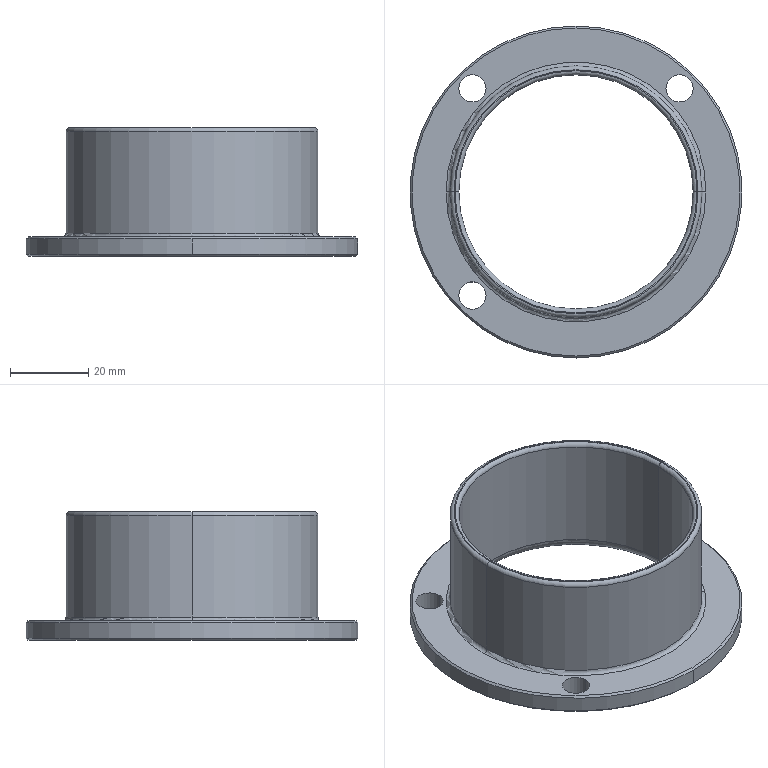Part | NX | features solid 2 | 1 solid | 27 faces | box 85 x 85 x 33 mm | volume 25500 mm3 | cylinder 12 | torus 8 | cone 4 | plane 3 | commonest cylinder face diameters 7 x6 60 x2 64.5 x2 85 x2
STEP:
#1=CARTESIAN_POINT('',(-450.,-1677.,947.));
#2=VERTEX_POINT('',#1);
#3=CARTESIAN_POINT('',(-450.,-1677.5,947.5));
#4=VERTEX_POINT('',#3);
#5=CARTESIAN_POINT('',(-450.,-1677.,947.));
#6=DIRECTION('',(0.,-0.7071,0.7071));
#7=VECTOR('',#6,1000.);
#8=LINE('',#5,#7);
#9=EDGE_CURVE('',#2,#4,#8,.T.);
#10=ORIENTED_EDGE('',*,*,#9,.F.);
#11=CARTESIAN_POINT('',(-450.,-1593.,947.));
#12=VERTEX_POINT('',#11);
#13=CARTESIAN_POINT('',(-450.,-1635.,947.));
#14=DIRECTION('',(0.,0.,-1.));
#15=DIRECTION('',(-1.,0.,0.));
#16=AXIS2_PLACEMENT_3D('',#13,#14,#15);
#17=CIRCLE('',#16,42.);
#18=EDGE_CURVE('',#12,#2,#17,.T.);
#19=ORIENTED_EDGE('',*,*,#18,.F.);
#20=CARTESIAN_POINT('',(-450.,-1592.5,947.5));
#21=VERTEX_POINT('',#20);
#22=CARTESIAN_POINT('',(-450.,-1593.,947.));
#23=DIRECTION('',(0.,0.7071,0.7071));
#24=VECTOR('',#23,1000.);
#25=LINE('',#22,#24);
#26=EDGE_CURVE('',#21,#12,#25,.F.);
#27=ORIENTED_EDGE('',*,*,#26,.F.);
#28=CARTESIAN_POINT('',(-450.,-1635.,947.5));
#29=DIRECTION('',(0.,0.,1.));
#30=DIRECTION('',(0.,-1.,0.));
#31=AXIS2_PLACEMENT_3D('',#28,#29,#30);
#32=CIRCLE('',#31,42.5);
#33=EDGE_CURVE('',#4,#21,#32,.T.);
#34=ORIENTED_EDGE('',*,*,#33,.F.);
#35=EDGE_LOOP('',(#10,#19,#27,#34));
#36=FACE_BOUND('',#35,.T.);
#37=CARTESIAN_POINT('',(-450.,-1635.,947.));
#38=DIRECTION('',(0.,0.,1.));
#39=DIRECTION('',(0.,1.,0.));
#40=AXIS2_PLACEMENT_3D('',#37,#38,#39);
#41=CONICAL_SURFACE('',#40,42.,0.7854);
#42=ADVANCED_FACE('',(#36),#41,.T.);
#43=CARTESIAN_POINT('',(-450.,-1593.,952.));
#44=VERTEX_POINT('',#43);
#45=CARTESIAN_POINT('',(-450.,-1592.5,951.5));
#46=VERTEX_POINT('',#45);
#47=CARTESIAN_POINT('',(-450.,-1592.5,951.5));
#48=DIRECTION('',(0.,0.7071,-0.7071));
#49=VECTOR('',#48,1000.);
#50=LINE('',#47,#49);
#51=EDGE_CURVE('',#44,#46,#50,.T.);
#52=ORIENTED_EDGE('',*,*,#51,.F.);
#53=CARTESIAN_POINT('',(-450.,-1677.,952.));
#54=VERTEX_POINT('',#53);
#55=CARTESIAN_POINT('',(-450.,-1635.,952.));
#56=DIRECTION('',(0.,0.,1.));
#57=DIRECTION('',(-1.,0.,0.));
#58=AXIS2_PLACEMENT_3D('',#55,#56,#57);
#59=CIRCLE('',#58,42.);
#60=EDGE_CURVE('',#54,#44,#59,.T.);
#61=ORIENTED_EDGE('',*,*,#60,.F.);
#62=CARTESIAN_POINT('',(-450.,-1677.5,951.5));
#63=VERTEX_POINT('',#62);
#64=CARTESIAN_POINT('',(-450.,-1677.5,951.5));
#65=DIRECTION('',(0.,-0.7071,-0.7071));
#66=VECTOR('',#65,1000.);
#67=LINE('',#64,#66);
#68=EDGE_CURVE('',#63,#54,#67,.F.);
#69=ORIENTED_EDGE('',*,*,#68,.F.);
#70=CARTESIAN_POINT('',(-450.,-1635.,951.5));
#71=DIRECTION('',(0.,0.,-1.));
#72=DIRECTION('',(0.,-1.,0.));
#73=AXIS2_PLACEMENT_3D('',#70,#71,#72);
#74=CIRCLE('',#73,42.5);
#75=EDGE_CURVE('',#46,#63,#74,.T.);
#76=ORIENTED_EDGE('',*,*,#75,.F.);
#77=EDGE_LOOP('',(#52,#61,#69,#76));
#78=FACE_BOUND('',#77,.T.);
#79=CARTESIAN_POINT('',(-450.,-1635.,951.5));
#80=DIRECTION('',(0.,0.,-1.));
#81=DIRECTION('',(0.,-1.,0.));
#82=AXIS2_PLACEMENT_3D('',#79,#80,#81);
#83=CONICAL_SURFACE('',#82,42.5,0.7854);
#84=ADVANCED_FACE('',(#78),#83,.T.);
#85=CARTESIAN_POINT('',(-417.75,-1635.,979.));
#86=VERTEX_POINT('',#85);
#87=CARTESIAN_POINT('',(-418.75,-1635.,980.));
#88=VERTEX_POINT('',#87);
#89=CARTESIAN_POINT('',(-418.75,-1635.,979.));
#90=DIRECTION('',(0.,1.,0.));
#91=DIRECTION('',(0.,0.,1.));
#92=AXIS2_PLACEMENT_3D('',#89,#90,#91);
#93=CIRCLE('',#92,1.);
#94=EDGE_CURVE('',#86,#88,#93,.F.);
#95=ORIENTED_EDGE('',*,*,#94,.T.);
#96=CARTESIAN_POINT('',(-481.25,-1635.,980.));
#97=VERTEX_POINT('',#96);
#98=CARTESIAN_POINT('',(-450.,-1635.,980.));
#99=DIRECTION('',(0.,0.,1.));
#100=DIRECTION('',(-1.,0.,0.));
#101=AXIS2_PLACEMENT_3D('',#98,#99,#100);
#102=CIRCLE('',#101,31.25);
#103=EDGE_CURVE('',#97,#88,#102,.T.);
#104=ORIENTED_EDGE('',*,*,#103,.F.);
#105=CARTESIAN_POINT('',(-482.25,-1635.,979.));
#106=VERTEX_POINT('',#105);
#107=CARTESIAN_POINT('',(-481.25,-1635.,979.));
#108=DIRECTION('',(0.,-1.,0.));
#109=DIRECTION('',(0.,0.,-1.));
#110=AXIS2_PLACEMENT_3D('',#107,#108,#109);
#111=CIRCLE('',#110,1.);
#112=EDGE_CURVE('',#97,#106,#111,.T.);
#113=ORIENTED_EDGE('',*,*,#112,.T.);
#114=CARTESIAN_POINT('',(-450.,-1635.,979.));
#115=DIRECTION('',(0.,0.,-1.));
#116=DIRECTION('',(-1.,0.,0.));
#117=AXIS2_PLACEMENT_3D('',#114,#115,#116);
#118=CIRCLE('',#117,32.25);
#119=EDGE_CURVE('',#86,#106,#118,.T.);
#120=ORIENTED_EDGE('',*,*,#119,.F.);
#121=EDGE_LOOP('',(#95,#104,#113,#120));
#122=FACE_BOUND('',#121,.T.);
#123=CARTESIAN_POINT('',(-450.,-1635.,979.));
#124=DIRECTION('',(0.,0.,-1.));
#125=DIRECTION('',(-1.,0.,0.));
#126=AXIS2_PLACEMENT_3D('',#123,#124,#125);
#127=TOROIDAL_SURFACE('',#126,31.25,1.);
#128=ADVANCED_FACE('',(#122),#127,.T.);
#129=CARTESIAN_POINT('',(-419.,-1635.,980.));
#130=VERTEX_POINT('',#129);
#131=CARTESIAN_POINT('',(-420.,-1635.,979.));
#132=VERTEX_POINT('',#131);
#133=CARTESIAN_POINT('',(-419.,-1635.,979.));
#134=DIRECTION('',(0.,1.,0.));
#135=DIRECTION('',(0.,0.,1.));
#136=AXIS2_PLACEMENT_3D('',#133,#134,#135);
#137=CIRCLE('',#136,1.);
#138=EDGE_CURVE('',#130,#132,#137,.F.);
#139=ORIENTED_EDGE('',*,*,#138,.T.);
#140=CARTESIAN_POINT('',(-480.,-1635.,979.));
#141=VERTEX_POINT('',#140);
#142=CARTESIAN_POINT('',(-450.,-1635.,979.));
#143=DIRECTION('',(0.,0.,1.));
#144=DIRECTION('',(-1.,0.,0.));
#145=AXIS2_PLACEMENT_3D('',#142,#143,#144);
#146=CIRCLE('',#145,30.);
#147=EDGE_CURVE('',#141,#132,#146,.T.);
#148=ORIENTED_EDGE('',*,*,#147,.F.);
#149=CARTESIAN_POINT('',(-481.,-1635.,980.));
#150=VERTEX_POINT('',#149);
#151=CARTESIAN_POINT('',(-481.,-1635.,979.));
#152=DIRECTION('',(0.,-1.,0.));
#153=DIRECTION('',(0.,0.,-1.));
#154=AXIS2_PLACEMENT_3D('',#151,#152,#153);
#155=CIRCLE('',#154,1.);
#156=EDGE_CURVE('',#141,#150,#155,.T.);
#157=ORIENTED_EDGE('',*,*,#156,.T.);
#158=CARTESIAN_POINT('',(-450.,-1635.,980.));
#159=DIRECTION('',(0.,0.,-1.));
#160=DIRECTION('',(-1.,0.,0.));
#161=AXIS2_PLACEMENT_3D('',#158,#159,#160);
#162=CIRCLE('',#161,31.);
#163=EDGE_CURVE('',#130,#150,#162,.T.);
#164=ORIENTED_EDGE('',*,*,#163,.F.);
#165=EDGE_LOOP('',(#139,#148,#157,#164));
#166=FACE_BOUND('',#165,.T.);
#167=CARTESIAN_POINT('',(-450.,-1635.,979.));
#168=DIRECTION('',(0.,0.,-1.));
#169=DIRECTION('',(-1.,0.,0.));
#170=AXIS2_PLACEMENT_3D('',#167,#168,#169);
#171=TOROIDAL_SURFACE('',#170,31.,1.);
#172=ADVANCED_FACE('',(#166),#171,.T.);
#173=CARTESIAN_POINT('',(-416.75,-1635.,952.));
#174=VERTEX_POINT('',#173);
#175=CARTESIAN_POINT('',(-417.75,-1635.,953.));
#176=VERTEX_POINT('',#175);
#177=CARTESIAN_POINT('',(-416.75,-1635.,953.));
#178=DIRECTION('',(0.,1.,0.));
#179=DIRECTION('',(0.,0.,1.));
#180=AXIS2_PLACEMENT_3D('',#177,#178,#179);
#181=CIRCLE('',#180,1.);
#182=EDGE_CURVE('',#174,#176,#181,.T.);
#183=ORIENTED_EDGE('',*,*,#182,.F.);
#184=CARTESIAN_POINT('',(-483.25,-1635.,952.));
#185=VERTEX_POINT('',#184);
#186=CARTESIAN_POINT('',(-450.,-1635.,952.));
#187=DIRECTION('',(0.,0.,-1.));
#188=DIRECTION('',(-1.,0.,0.));
#189=AXIS2_PLACEMENT_3D('',#186,#187,#188);
#190=CIRCLE('',#189,33.25);
#191=EDGE_CURVE('',#185,#174,#190,.T.);
#192=ORIENTED_EDGE('',*,*,#191,.F.);
#193=CARTESIAN_POINT('',(-482.25,-1635.,953.));
#194=VERTEX_POINT('',#193);
#195=CARTESIAN_POINT('',(-483.25,-1635.,953.));
#196=DIRECTION('',(0.,-1.,0.));
#197=DIRECTION('',(0.,0.,-1.));
#198=AXIS2_PLACEMENT_3D('',#195,#196,#197);
#199=CIRCLE('',#198,1.);
#200=EDGE_CURVE('',#194,#185,#199,.F.);
#201=ORIENTED_EDGE('',*,*,#200,.F.);
#202=CARTESIAN_POINT('',(-450.,-1635.,953.));
#203=DIRECTION('',(0.,0.,1.));
#204=DIRECTION('',(-1.,0.,0.));
#205=AXIS2_PLACEMENT_3D('',#202,#203,#204);
#206=CIRCLE('',#205,32.25);
#207=EDGE_CURVE('',#176,#194,#206,.T.);
#208=ORIENTED_EDGE('',*,*,#207,.F.);
#209=EDGE_LOOP('',(#183,#192,#201,#208));
#210=FACE_BOUND('',#209,.T.);
#211=CARTESIAN_POINT('',(-450.,-1635.,953.));
#212=DIRECTION('',(0.,0.,-1.));
#213=DIRECTION('',(-1.,0.,0.));
#214=AXIS2_PLACEMENT_3D('',#211,#212,#213);
#215=TOROIDAL_SURFACE('',#214,33.25,1.);
#216=ADVANCED_FACE('',(#210),#215,.F.);
#217=CARTESIAN_POINT('',(-420.,-1635.,950.));
#218=VERTEX_POINT('',#217);
#219=CARTESIAN_POINT('',(-417.,-1635.,947.));
#220=VERTEX_POINT('',#219);
#221=CARTESIAN_POINT('',(-417.,-1635.,950.));
#222=DIRECTION('',(0.,1.,0.));
#223=DIRECTION('',(0.,0.,1.));
#224=AXIS2_PLACEMENT_3D('',#221,#222,#223);
#225=CIRCLE('',#224,3.);
#226=EDGE_CURVE('',#218,#220,#225,.F.);
#227=ORIENTED_EDGE('',*,*,#226,.T.);
#228=CARTESIAN_POINT('',(-483.,-1635.,947.));
#229=VERTEX_POINT('',#228);
#230=CARTESIAN_POINT('',(-450.,-1635.,947.));
#231=DIRECTION('',(0.,0.,1.));
#232=DIRECTION('',(-1.,0.,0.));
#233=AXIS2_PLACEMENT_3D('',#230,#231,#232);
#234=CIRCLE('',#233,33.);
#235=EDGE_CURVE('',#229,#220,#234,.T.);
#236=ORIENTED_EDGE('',*,*,#235,.F.);
#237=CARTESIAN_POINT('',(-480.,-1635.,950.));
#238=VERTEX_POINT('',#237);
#239=CARTESIAN_POINT('',(-483.,-1635.,950.));
#240=DIRECTION('',(0.,-1.,0.));
#241=DIRECTION('',(0.,0.,-1.));
#242=AXIS2_PLACEMENT_3D('',#239,#240,#241);
#243=CIRCLE('',#242,3.);
#244=EDGE_CURVE('',#229,#238,#243,.T.);
#245=ORIENTED_EDGE('',*,*,#244,.T.);
#246=CARTESIAN_POINT('',(-450.,-1635.,950.));
#247=DIRECTION('',(0.,0.,-1.));
#248=DIRECTION('',(-1.,0.,0.));
#249=AXIS2_PLACEMENT_3D('',#246,#247,#248);
#250=CIRCLE('',#249,30.);
#251=EDGE_CURVE('',#218,#238,#250,.T.);
#252=ORIENTED_EDGE('',*,*,#251,.F.);
#253=EDGE_LOOP('',(#227,#236,#245,#252));
#254=FACE_BOUND('',#253,.T.);
#255=CARTESIAN_POINT('',(-450.,-1635.,950.));
#256=DIRECTION('',(0.,0.,-1.));
#257=DIRECTION('',(-1.,0.,0.));
#258=AXIS2_PLACEMENT_3D('',#255,#256,#257);
#259=TOROIDAL_SURFACE('',#258,33.,3.);
#260=ADVANCED_FACE('',(#254),#259,.T.);
#261=CARTESIAN_POINT('',(-426.983,-1608.483,952.));
#262=VERTEX_POINT('',#261);
#263=CARTESIAN_POINT('',(-426.983,-1608.483,947.));
#264=VERTEX_POINT('',#263);
#265=CARTESIAN_POINT('',(-426.983,-1608.483,827.344));
#266=DIRECTION('',(0.,0.,1.));
#267=VECTOR('',#266,1000.);
#268=LINE('',#265,#267);
#269=EDGE_CURVE('',#262,#264,#268,.F.);
#270=ORIENTED_EDGE('',*,*,#269,.T.);
#271=CARTESIAN_POINT('',(-419.983,-1608.483,947.));
#272=VERTEX_POINT('',#271);
#273=CARTESIAN_POINT('',(-423.483,-1608.483,947.));
#274=DIRECTION('',(0.,0.,-1.));
#275=DIRECTION('',(-1.,0.,0.));
#276=AXIS2_PLACEMENT_3D('',#273,#274,#275);
#277=CIRCLE('',#276,3.5);
#278=EDGE_CURVE('',#264,#272,#277,.T.);
#279=ORIENTED_EDGE('',*,*,#278,.T.);
#280=CARTESIAN_POINT('',(-419.983,-1608.483,952.));
#281=VERTEX_POINT('',#280);
#282=CARTESIAN_POINT('',(-419.983,-1608.483,827.344));
#283=DIRECTION('',(0.,0.,1.));
#284=VECTOR('',#283,1000.);
#285=LINE('',#282,#284);
#286=EDGE_CURVE('',#272,#281,#285,.T.);
#287=ORIENTED_EDGE('',*,*,#286,.T.);
#288=CARTESIAN_POINT('',(-423.483,-1608.483,952.));
#289=DIRECTION('',(0.,0.,1.));
#290=DIRECTION('',(0.,1.,0.));
#291=AXIS2_PLACEMENT_3D('',#288,#289,#290);
#292=CIRCLE('',#291,3.5);
#293=EDGE_CURVE('',#281,#262,#292,.T.);
#294=ORIENTED_EDGE('',*,*,#293,.T.);
#295=EDGE_LOOP('',(#270,#279,#287,#294));
#296=FACE_BOUND('',#295,.T.);
#297=CARTESIAN_POINT('',(-423.483,-1608.483,827.344));
#298=DIRECTION('',(0.,0.,1.));
#299=DIRECTION('',(1.,0.,0.));
#300=AXIS2_PLACEMENT_3D('',#297,#298,#299);
#301=CYLINDRICAL_SURFACE('',#300,3.5);
#302=ADVANCED_FACE('',(#296),#301,.F.);
#303=CARTESIAN_POINT('',(-480.017,-1608.483,947.));
#304=VERTEX_POINT('',#303);
#305=CARTESIAN_POINT('',(-480.017,-1608.483,952.));
#306=VERTEX_POINT('',#305);
#307=CARTESIAN_POINT('',(-480.017,-1608.483,827.344));
#308=DIRECTION('',(0.,0.,1.));
#309=VECTOR('',#308,1000.);
#310=LINE('',#307,#309);
#311=EDGE_CURVE('',#304,#306,#310,.T.);
#312=ORIENTED_EDGE('',*,*,#311,.F.);
#313=CARTESIAN_POINT('',(-473.017,-1608.483,947.));
#314=VERTEX_POINT('',#313);
#315=CARTESIAN_POINT('',(-476.517,-1608.483,947.));
#316=DIRECTION('',(0.,0.,-1.));
#317=DIRECTION('',(-1.,0.,0.));
#318=AXIS2_PLACEMENT_3D('',#315,#316,#317);
#319=CIRCLE('',#318,3.5);
#320=EDGE_CURVE('',#304,#314,#319,.T.);
#321=ORIENTED_EDGE('',*,*,#320,.T.);
#322=CARTESIAN_POINT('',(-473.017,-1608.483,952.));
#323=VERTEX_POINT('',#322);
#324=CARTESIAN_POINT('',(-473.017,-1608.483,827.344));
#325=DIRECTION('',(0.,0.,1.));
#326=VECTOR('',#325,1000.);
#327=LINE('',#324,#326);
#328=EDGE_CURVE('',#323,#314,#327,.F.);
#329=ORIENTED_EDGE('',*,*,#328,.F.);
#330=CARTESIAN_POINT('',(-476.517,-1608.483,952.));
#331=DIRECTION('',(0.,0.,1.));
#332=DIRECTION('',(0.,1.,0.));
#333=AXIS2_PLACEMENT_3D('',#330,#331,#332);
#334=CIRCLE('',#333,3.5);
#335=EDGE_CURVE('',#323,#306,#334,.T.);
#336=ORIENTED_EDGE('',*,*,#335,.T.);
#337=EDGE_LOOP('',(#312,#321,#329,#336));
#338=FACE_BOUND('',#337,.T.);
#339=CARTESIAN_POINT('',(-476.517,-1608.483,827.344));
#340=DIRECTION('',(0.,0.,1.));
#341=DIRECTION('',(1.,0.,0.));
#342=AXIS2_PLACEMENT_3D('',#339,#340,#341);
#343=CYLINDRICAL_SURFACE('',#342,3.5);
#344=ADVANCED_FACE('',(#338),#343,.F.);
#345=CARTESIAN_POINT('',(-480.017,-1661.517,947.));
#346=VERTEX_POINT('',#345);
#347=CARTESIAN_POINT('',(-480.017,-1661.517,952.));
#348=VERTEX_POINT('',#347);
#349=CARTESIAN_POINT('',(-480.017,-1661.517,827.344));
#350=DIRECTION('',(0.,0.,1.));
#351=VECTOR('',#350,1000.);
#352=LINE('',#349,#351);
#353=EDGE_CURVE('',#346,#348,#352,.T.);
#354=ORIENTED_EDGE('',*,*,#353,.F.);
#355=CARTESIAN_POINT('',(-473.017,-1661.517,947.));
#356=VERTEX_POINT('',#355);
#357=CARTESIAN_POINT('',(-476.517,-1661.517,947.));
#358=DIRECTION('',(0.,0.,-1.));
#359=DIRECTION('',(-1.,0.,0.));
#360=AXIS2_PLACEMENT_3D('',#357,#358,#359);
#361=CIRCLE('',#360,3.5);
#362=EDGE_CURVE('',#346,#356,#361,.T.);
#363=ORIENTED_EDGE('',*,*,#362,.T.);
#364=CARTESIAN_POINT('',(-473.017,-1661.517,952.));
#365=VERTEX_POINT('',#364);
#366=CARTESIAN_POINT('',(-473.017,-1661.517,827.344));
#367=DIRECTION('',(0.,0.,1.));
#368=VECTOR('',#367,1000.);
#369=LINE('',#366,#368);
#370=EDGE_CURVE('',#365,#356,#369,.F.);
#371=ORIENTED_EDGE('',*,*,#370,.F.);
#372=CARTESIAN_POINT('',(-476.517,-1661.517,952.));
#373=DIRECTION('',(0.,0.,1.));
#374=DIRECTION('',(0.,1.,0.));
#375=AXIS2_PLACEMENT_3D('',#372,#373,#374);
#376=CIRCLE('',#375,3.5);
#377=EDGE_CURVE('',#365,#348,#376,.T.);
#378=ORIENTED_EDGE('',*,*,#377,.T.);
#379=EDGE_LOOP('',(#354,#363,#371,#378));
#380=FACE_BOUND('',#379,.T.);
#381=CARTESIAN_POINT('',(-476.517,-1661.517,827.344));
#382=DIRECTION('',(0.,0.,1.));
#383=DIRECTION('',(1.,0.,0.));
#384=AXIS2_PLACEMENT_3D('',#381,#382,#383);
#385=CYLINDRICAL_SURFACE('',#384,3.5);
#386=ADVANCED_FACE('',(#380),#385,.F.);
#387=CARTESIAN_POINT('',(-480.,-1635.,980.));
#388=DIRECTION('',(0.,0.,-1.));
#389=VECTOR('',#388,1000.);
#390=LINE('',#387,#389);
#391=EDGE_CURVE('',#238,#141,#390,.F.);
#392=ORIENTED_EDGE('',*,*,#391,.T.);
#393=ORIENTED_EDGE('',*,*,#147,.T.);
#394=CARTESIAN_POINT('',(-420.,-1635.,980.));
#395=DIRECTION('',(0.,0.,-1.));
#396=VECTOR('',#395,1000.);
#397=LINE('',#394,#396);
#398=EDGE_CURVE('',#132,#218,#397,.T.);
#399=ORIENTED_EDGE('',*,*,#398,.T.);
#400=ORIENTED_EDGE('',*,*,#251,.T.);
#401=EDGE_LOOP('',(#392,#393,#399,#400));
#402=FACE_BOUND('',#401,.T.);
#403=CARTESIAN_POINT('',(-450.,-1635.,980.));
#404=DIRECTION('',(0.,0.,-1.));
#405=DIRECTION('',(1.,0.,0.));
#406=AXIS2_PLACEMENT_3D('',#403,#404,#405);
#407=CYLINDRICAL_SURFACE('',#406,30.);
#408=ADVANCED_FACE('',(#402),#407,.F.);
#409=CARTESIAN_POINT('',(-450.,-1635.,980.));
#410=DIRECTION('',(0.,0.,-1.));
#411=DIRECTION('',(-1.,0.,0.));
#412=AXIS2_PLACEMENT_3D('',#409,#410,#411);
#413=CIRCLE('',#412,31.);
#414=EDGE_CURVE('',#150,#130,#413,.T.);
#415=ORIENTED_EDGE('',*,*,#414,.T.);
#416=ORIENTED_EDGE('',*,*,#163,.T.);
#417=EDGE_LOOP('',(#415,#416));
#418=FACE_BOUND('',#417,.T.);
#419=ORIENTED_EDGE('',*,*,#103,.T.);
#420=CARTESIAN_POINT('',(-450.,-1635.,980.));
#421=DIRECTION('',(0.,0.,1.));
#422=DIRECTION('',(-1.,0.,0.));
#423=AXIS2_PLACEMENT_3D('',#420,#421,#422);
#424=CIRCLE('',#423,31.25);
#425=EDGE_CURVE('',#88,#97,#424,.T.);
#426=ORIENTED_EDGE('',*,*,#425,.T.);
#427=EDGE_LOOP('',(#419,#426));
#428=FACE_BOUND('',#427,.T.);
#429=CARTESIAN_POINT('',(-450.,-1635.,980.));
#430=DIRECTION('',(0.,0.,-1.));
#431=DIRECTION('',(0.,-1.,0.));
#432=AXIS2_PLACEMENT_3D('',#429,#430,#431);
#433=PLANE('',#432);
#434=ADVANCED_FACE('',(#418,#428),#433,.F.);
#435=CARTESIAN_POINT('',(-417.75,-1635.,980.));
#436=DIRECTION('',(0.,0.,-1.));
#437=VECTOR('',#436,1000.);
#438=LINE('',#435,#437);
#439=EDGE_CURVE('',#176,#86,#438,.F.);
#440=ORIENTED_EDGE('',*,*,#439,.T.);
#441=ORIENTED_EDGE('',*,*,#119,.T.);
#442=CARTESIAN_POINT('',(-482.25,-1635.,980.));
#443=DIRECTION('',(0.,0.,-1.));
#444=VECTOR('',#443,1000.);
#445=LINE('',#442,#444);
#446=EDGE_CURVE('',#106,#194,#445,.T.);
#447=ORIENTED_EDGE('',*,*,#446,.T.);
#448=CARTESIAN_POINT('',(-450.,-1635.,953.));
#449=DIRECTION('',(0.,0.,1.));
#450=DIRECTION('',(-1.,0.,0.));
#451=AXIS2_PLACEMENT_3D('',#448,#449,#450);
#452=CIRCLE('',#451,32.25);
#453=EDGE_CURVE('',#194,#176,#452,.T.);
#454=ORIENTED_EDGE('',*,*,#453,.T.);
#455=EDGE_LOOP('',(#440,#441,#447,#454));
#456=FACE_BOUND('',#455,.T.);
#457=CARTESIAN_POINT('',(-450.,-1635.,980.));
#458=DIRECTION('',(0.,0.,-1.));
#459=DIRECTION('',(-1.,0.,0.));
#460=AXIS2_PLACEMENT_3D('',#457,#458,#459);
#461=CYLINDRICAL_SURFACE('',#460,32.25);
#462=ADVANCED_FACE('',(#456),#461,.T.);
#463=CARTESIAN_POINT('',(-476.517,-1661.517,947.));
#464=DIRECTION('',(0.,0.,-1.));
#465=DIRECTION('',(-1.,0.,0.));
#466=AXIS2_PLACEMENT_3D('',#463,#464,#465);
#467=CIRCLE('',#466,3.5);
#468=EDGE_CURVE('',#356,#346,#467,.T.);
#469=ORIENTED_EDGE('',*,*,#468,.F.);
#470=ORIENTED_EDGE('',*,*,#362,.F.);
#471=EDGE_LOOP('',(#469,#470));
#472=FACE_BOUND('',#471,.T.);
#473=CARTESIAN_POINT('',(-476.517,-1608.483,947.));
#474=DIRECTION('',(0.,0.,-1.));
#475=DIRECTION('',(-1.,0.,0.));
#476=AXIS2_PLACEMENT_3D('',#473,#474,#475);
#477=CIRCLE('',#476,3.5);
#478=EDGE_CURVE('',#314,#304,#477,.T.);
#479=ORIENTED_EDGE('',*,*,#478,.F.);
#480=ORIENTED_EDGE('',*,*,#320,.F.);
#481=EDGE_LOOP('',(#479,#480));
#482=FACE_BOUND('',#481,.T.);
#483=CARTESIAN_POINT('',(-423.483,-1608.483,947.));
#484=DIRECTION('',(0.,0.,-1.));
#485=DIRECTION('',(-1.,0.,0.));
#486=AXIS2_PLACEMENT_3D('',#483,#484,#485);
#487=CIRCLE('',#486,3.5);
#488=EDGE_CURVE('',#272,#264,#487,.T.);
#489=ORIENTED_EDGE('',*,*,#488,.F.);
#490=ORIENTED_EDGE('',*,*,#278,.F.);
#491=EDGE_LOOP('',(#489,#490));
#492=FACE_BOUND('',#491,.T.);
#493=ORIENTED_EDGE('',*,*,#235,.T.);
#494=CARTESIAN_POINT('',(-450.,-1635.,947.));
#495=DIRECTION('',(0.,0.,1.));
#496=DIRECTION('',(-1.,0.,0.));
#497=AXIS2_PLACEMENT_3D('',#494,#495,#496);
#498=CIRCLE('',#497,33.);
#499=EDGE_CURVE('',#220,#229,#498,.T.);
#500=ORIENTED_EDGE('',*,*,#499,.T.);
#501=EDGE_LOOP('',(#493,#500));
#502=FACE_BOUND('',#501,.T.);
#503=ORIENTED_EDGE('',*,*,#18,.T.);
#504=CARTESIAN_POINT('',(-450.,-1635.,947.));
#505=DIRECTION('',(0.,0.,-1.));
#506=DIRECTION('',(-1.,0.,0.));
#507=AXIS2_PLACEMENT_3D('',#504,#505,#506);
#508=CIRCLE('',#507,42.);
#509=EDGE_CURVE('',#2,#12,#508,.T.);
#510=ORIENTED_EDGE('',*,*,#509,.T.);
#511=EDGE_LOOP('',(#503,#510));
#512=FACE_BOUND('',#511,.T.);
#513=CARTESIAN_POINT('',(-450.,-1635.,947.));
#514=DIRECTION('',(0.,0.,-1.));
#515=DIRECTION('',(0.,-1.,0.));
#516=AXIS2_PLACEMENT_3D('',#513,#514,#515);
#517=PLANE('',#516);
#518=ADVANCED_FACE('',(#472,#482,#492,#502,#512),#517,.T.);
#519=ORIENTED_EDGE('',*,*,#377,.F.);
#520=CARTESIAN_POINT('',(-476.517,-1661.517,952.));
#521=DIRECTION('',(0.,0.,1.));
#522=DIRECTION('',(0.,1.,0.));
#523=AXIS2_PLACEMENT_3D('',#520,#521,#522);
#524=CIRCLE('',#523,3.5);
#525=EDGE_CURVE('',#348,#365,#524,.T.);
#526=ORIENTED_EDGE('',*,*,#525,.F.);
#527=EDGE_LOOP('',(#519,#526));
#528=FACE_BOUND('',#527,.T.);
#529=ORIENTED_EDGE('',*,*,#335,.F.);
#530=CARTESIAN_POINT('',(-476.517,-1608.483,952.));
#531=DIRECTION('',(0.,0.,1.));
#532=DIRECTION('',(0.,1.,0.));
#533=AXIS2_PLACEMENT_3D('',#530,#531,#532);
#534=CIRCLE('',#533,3.5);
#535=EDGE_CURVE('',#306,#323,#534,.T.);
#536=ORIENTED_EDGE('',*,*,#535,.F.);
#537=EDGE_LOOP('',(#529,#536));
#538=FACE_BOUND('',#537,.T.);
#539=ORIENTED_EDGE('',*,*,#293,.F.);
#540=CARTESIAN_POINT('',(-423.483,-1608.483,952.));
#541=DIRECTION('',(0.,0.,1.));
#542=DIRECTION('',(0.,1.,0.));
#543=AXIS2_PLACEMENT_3D('',#540,#541,#542);
#544=CIRCLE('',#543,3.5);
#545=EDGE_CURVE('',#262,#281,#544,.T.);
#546=ORIENTED_EDGE('',*,*,#545,.F.);
#547=EDGE_LOOP('',(#539,#546));
#548=FACE_BOUND('',#547,.T.);
#549=ORIENTED_EDGE('',*,*,#191,.T.);
#550=CARTESIAN_POINT('',(-450.,-1635.,952.));
#551=DIRECTION('',(0.,0.,-1.));
#552=DIRECTION('',(-1.,0.,0.));
#553=AXIS2_PLACEMENT_3D('',#550,#551,#552);
#554=CIRCLE('',#553,33.25);
#555=EDGE_CURVE('',#174,#185,#554,.T.);
#556=ORIENTED_EDGE('',*,*,#555,.T.);
#557=EDGE_LOOP('',(#549,#556));
#558=FACE_BOUND('',#557,.T.);
#559=ORIENTED_EDGE('',*,*,#60,.T.);
#560=CARTESIAN_POINT('',(-450.,-1635.,952.));
#561=DIRECTION('',(0.,0.,1.));
#562=DIRECTION('',(-1.,0.,0.));
#563=AXIS2_PLACEMENT_3D('',#560,#561,#562);
#564=CIRCLE('',#563,42.);
#565=EDGE_CURVE('',#44,#54,#564,.T.);
#566=ORIENTED_EDGE('',*,*,#565,.T.);
#567=EDGE_LOOP('',(#559,#566));
#568=FACE_BOUND('',#567,.T.);
#569=CARTESIAN_POINT('',(-450.,-1635.,952.));
#570=DIRECTION('',(0.,0.,-1.));
#571=DIRECTION('',(0.,-1.,0.));
#572=AXIS2_PLACEMENT_3D('',#569,#570,#571);
#573=PLANE('',#572);
#574=ADVANCED_FACE('',(#528,#538,#548,#558,#568),#573,.F.);
#575=CARTESIAN_POINT('',(-450.,-1592.5,952.));
#576=DIRECTION('',(0.,0.,-1.));
#577=VECTOR('',#576,1000.);
#578=LINE('',#575,#577);
#579=EDGE_CURVE('',#46,#21,#578,.T.);
#580=ORIENTED_EDGE('',*,*,#579,.F.);
#581=ORIENTED_EDGE('',*,*,#75,.T.);
#582=CARTESIAN_POINT('',(-450.,-1677.5,952.));
#583=DIRECTION('',(0.,0.,-1.));
#584=VECTOR('',#583,1000.);
#585=LINE('',#582,#584);
#586=EDGE_CURVE('',#4,#63,#585,.F.);
#587=ORIENTED_EDGE('',*,*,#586,.F.);
#588=ORIENTED_EDGE('',*,*,#33,.T.);
#589=EDGE_LOOP('',(#580,#581,#587,#588));
#590=FACE_BOUND('',#589,.T.);
#591=CARTESIAN_POINT('',(-450.,-1635.,952.));
#592=DIRECTION('',(0.,0.,-1.));
#593=DIRECTION('',(0.,-1.,0.));
#594=AXIS2_PLACEMENT_3D('',#591,#592,#593);
#595=CYLINDRICAL_SURFACE('',#594,42.5);
#596=ADVANCED_FACE('',(#590),#595,.T.);
#597=CARTESIAN_POINT('',(-450.,-1635.,951.5));
#598=DIRECTION('',(0.,0.,-1.));
#599=DIRECTION('',(0.,-1.,0.));
#600=AXIS2_PLACEMENT_3D('',#597,#598,#599);
#601=CIRCLE('',#600,42.5);
#602=EDGE_CURVE('',#63,#46,#601,.T.);
#603=ORIENTED_EDGE('',*,*,#602,.T.);
#604=ORIENTED_EDGE('',*,*,#579,.T.);
#605=CARTESIAN_POINT('',(-450.,-1635.,947.5));
#606=DIRECTION('',(0.,0.,1.));
#607=DIRECTION('',(0.,-1.,0.));
#608=AXIS2_PLACEMENT_3D('',#605,#606,#607);
#609=CIRCLE('',#608,42.5);
#610=EDGE_CURVE('',#21,#4,#609,.T.);
#611=ORIENTED_EDGE('',*,*,#610,.T.);
#612=ORIENTED_EDGE('',*,*,#586,.T.);
#613=EDGE_LOOP('',(#603,#604,#611,#612));
#614=FACE_BOUND('',#613,.T.);
#615=CARTESIAN_POINT('',(-450.,-1635.,952.));
#616=DIRECTION('',(0.,0.,-1.));
#617=DIRECTION('',(0.,-1.,0.));
#618=AXIS2_PLACEMENT_3D('',#615,#616,#617);
#619=CYLINDRICAL_SURFACE('',#618,42.5);
#620=ADVANCED_FACE('',(#614),#619,.T.);
#621=CARTESIAN_POINT('',(-450.,-1635.,979.));
#622=DIRECTION('',(0.,0.,-1.));
#623=DIRECTION('',(-1.,0.,0.));
#624=AXIS2_PLACEMENT_3D('',#621,#622,#623);
#625=CIRCLE('',#624,32.25);
#626=EDGE_CURVE('',#106,#86,#625,.T.);
#627=ORIENTED_EDGE('',*,*,#626,.T.);
#628=ORIENTED_EDGE('',*,*,#439,.F.);
#629=ORIENTED_EDGE('',*,*,#207,.T.);
#630=ORIENTED_EDGE('',*,*,#446,.F.);
#631=EDGE_LOOP('',(#627,#628,#629,#630));
#632=FACE_BOUND('',#631,.T.);
#633=CARTESIAN_POINT('',(-450.,-1635.,980.));
#634=DIRECTION('',(0.,0.,-1.));
#635=DIRECTION('',(-1.,0.,0.));
#636=AXIS2_PLACEMENT_3D('',#633,#634,#635);
#637=CYLINDRICAL_SURFACE('',#636,32.25);
#638=ADVANCED_FACE('',(#632),#637,.T.);
#639=CARTESIAN_POINT('',(-450.,-1635.,979.));
#640=DIRECTION('',(0.,0.,1.));
#641=DIRECTION('',(-1.,0.,0.));
#642=AXIS2_PLACEMENT_3D('',#639,#640,#641);
#643=CIRCLE('',#642,30.);
#644=EDGE_CURVE('',#132,#141,#643,.T.);
#645=ORIENTED_EDGE('',*,*,#644,.T.);
#646=ORIENTED_EDGE('',*,*,#391,.F.);
#647=CARTESIAN_POINT('',(-450.,-1635.,950.));
#648=DIRECTION('',(0.,0.,-1.));
#649=DIRECTION('',(-1.,0.,0.));
#650=AXIS2_PLACEMENT_3D('',#647,#648,#649);
#651=CIRCLE('',#650,30.);
#652=EDGE_CURVE('',#238,#218,#651,.T.);
#653=ORIENTED_EDGE('',*,*,#652,.T.);
#654=ORIENTED_EDGE('',*,*,#398,.F.);
#655=EDGE_LOOP('',(#645,#646,#653,#654));
#656=FACE_BOUND('',#655,.T.);
#657=CARTESIAN_POINT('',(-450.,-1635.,980.));
#658=DIRECTION('',(0.,0.,-1.));
#659=DIRECTION('',(1.,0.,0.));
#660=AXIS2_PLACEMENT_3D('',#657,#658,#659);
#661=CYLINDRICAL_SURFACE('',#660,30.);
#662=ADVANCED_FACE('',(#656),#661,.F.);
#663=ORIENTED_EDGE('',*,*,#468,.T.);
#664=ORIENTED_EDGE('',*,*,#353,.T.);
#665=ORIENTED_EDGE('',*,*,#525,.T.);
#666=ORIENTED_EDGE('',*,*,#370,.T.);
#667=EDGE_LOOP('',(#663,#664,#665,#666));
#668=FACE_BOUND('',#667,.T.);
#669=CARTESIAN_POINT('',(-476.517,-1661.517,827.344));
#670=DIRECTION('',(0.,0.,1.));
#671=DIRECTION('',(1.,0.,0.));
#672=AXIS2_PLACEMENT_3D('',#669,#670,#671);
#673=CYLINDRICAL_SURFACE('',#672,3.5);
#674=ADVANCED_FACE('',(#668),#673,.F.);
#675=ORIENTED_EDGE('',*,*,#478,.T.);
#676=ORIENTED_EDGE('',*,*,#311,.T.);
#677=ORIENTED_EDGE('',*,*,#535,.T.);
#678=ORIENTED_EDGE('',*,*,#328,.T.);
#679=EDGE_LOOP('',(#675,#676,#677,#678));
#680=FACE_BOUND('',#679,.T.);
#681=CARTESIAN_POINT('',(-476.517,-1608.483,827.344));
#682=DIRECTION('',(0.,0.,1.));
#683=DIRECTION('',(1.,0.,0.));
#684=AXIS2_PLACEMENT_3D('',#681,#682,#683);
#685=CYLINDRICAL_SURFACE('',#684,3.5);
#686=ADVANCED_FACE('',(#680),#685,.F.);
#687=ORIENTED_EDGE('',*,*,#488,.T.);
#688=ORIENTED_EDGE('',*,*,#269,.F.);
#689=ORIENTED_EDGE('',*,*,#545,.T.);
#690=ORIENTED_EDGE('',*,*,#286,.F.);
#691=EDGE_LOOP('',(#687,#688,#689,#690));
#692=FACE_BOUND('',#691,.T.);
#693=CARTESIAN_POINT('',(-423.483,-1608.483,827.344));
#694=DIRECTION('',(0.,0.,1.));
#695=DIRECTION('',(1.,0.,0.));
#696=AXIS2_PLACEMENT_3D('',#693,#694,#695);
#697=CYLINDRICAL_SURFACE('',#696,3.5);
#698=ADVANCED_FACE('',(#692),#697,.F.);
#699=ORIENTED_EDGE('',*,*,#499,.F.);
#700=ORIENTED_EDGE('',*,*,#226,.F.);
#701=ORIENTED_EDGE('',*,*,#652,.F.);
#702=ORIENTED_EDGE('',*,*,#244,.F.);
#703=EDGE_LOOP('',(#699,#700,#701,#702));
#704=FACE_BOUND('',#703,.T.);
#705=CARTESIAN_POINT('',(-450.,-1635.,950.));
#706=DIRECTION('',(0.,0.,-1.));
#707=DIRECTION('',(-1.,0.,0.));
#708=AXIS2_PLACEMENT_3D('',#705,#706,#707);
#709=TOROIDAL_SURFACE('',#708,33.,3.);
#710=ADVANCED_FACE('',(#704),#709,.T.);
#711=ORIENTED_EDGE('',*,*,#555,.F.);
#712=ORIENTED_EDGE('',*,*,#182,.T.);
#713=ORIENTED_EDGE('',*,*,#453,.F.);
#714=ORIENTED_EDGE('',*,*,#200,.T.);
#715=EDGE_LOOP('',(#711,#712,#713,#714));
#716=FACE_BOUND('',#715,.T.);
#717=CARTESIAN_POINT('',(-450.,-1635.,953.));
#718=DIRECTION('',(0.,0.,-1.));
#719=DIRECTION('',(-1.,0.,0.));
#720=AXIS2_PLACEMENT_3D('',#717,#718,#719);
#721=TOROIDAL_SURFACE('',#720,33.25,1.);
#722=ADVANCED_FACE('',(#716),#721,.F.);
#723=ORIENTED_EDGE('',*,*,#644,.F.);
#724=ORIENTED_EDGE('',*,*,#138,.F.);
#725=ORIENTED_EDGE('',*,*,#414,.F.);
#726=ORIENTED_EDGE('',*,*,#156,.F.);
#727=EDGE_LOOP('',(#723,#724,#725,#726));
#728=FACE_BOUND('',#727,.T.);
#729=CARTESIAN_POINT('',(-450.,-1635.,979.));
#730=DIRECTION('',(0.,0.,-1.));
#731=DIRECTION('',(-1.,0.,0.));
#732=AXIS2_PLACEMENT_3D('',#729,#730,#731);
#733=TOROIDAL_SURFACE('',#732,31.,1.);
#734=ADVANCED_FACE('',(#728),#733,.T.);
#735=ORIENTED_EDGE('',*,*,#425,.F.);
#736=ORIENTED_EDGE('',*,*,#94,.F.);
#737=ORIENTED_EDGE('',*,*,#626,.F.);
#738=ORIENTED_EDGE('',*,*,#112,.F.);
#739=EDGE_LOOP('',(#735,#736,#737,#738));
#740=FACE_BOUND('',#739,.T.);
#741=CARTESIAN_POINT('',(-450.,-1635.,979.));
#742=DIRECTION('',(0.,0.,-1.));
#743=DIRECTION('',(-1.,0.,0.));
#744=AXIS2_PLACEMENT_3D('',#741,#742,#743);
#745=TOROIDAL_SURFACE('',#744,31.25,1.);
#746=ADVANCED_FACE('',(#740),#745,.T.);
#747=ORIENTED_EDGE('',*,*,#565,.F.);
#748=ORIENTED_EDGE('',*,*,#51,.T.);
#749=ORIENTED_EDGE('',*,*,#602,.F.);
#750=ORIENTED_EDGE('',*,*,#68,.T.);
#751=EDGE_LOOP('',(#747,#748,#749,#750));
#752=FACE_BOUND('',#751,.T.);
#753=CARTESIAN_POINT('',(-450.,-1635.,951.5));
#754=DIRECTION('',(0.,0.,-1.));
#755=DIRECTION('',(0.,-1.,0.));
#756=AXIS2_PLACEMENT_3D('',#753,#754,#755);
#757=CONICAL_SURFACE('',#756,42.5,0.7854);
#758=ADVANCED_FACE('',(#752),#757,.T.);
#759=ORIENTED_EDGE('',*,*,#509,.F.);
#760=ORIENTED_EDGE('',*,*,#9,.T.);
#761=ORIENTED_EDGE('',*,*,#610,.F.);
#762=ORIENTED_EDGE('',*,*,#26,.T.);
#763=EDGE_LOOP('',(#759,#760,#761,#762));
#764=FACE_BOUND('',#763,.T.);
#765=CARTESIAN_POINT('',(-450.,-1635.,947.));
#766=DIRECTION('',(0.,0.,1.));
#767=DIRECTION('',(0.,1.,0.));
#768=AXIS2_PLACEMENT_3D('',#765,#766,#767);
#769=CONICAL_SURFACE('',#768,42.,0.7854);
#770=ADVANCED_FACE('',(#764),#769,.T.);
#771=CLOSED_SHELL('',(#42,#84,#128,#172,#216,#260,#302,#344,#386,#408,#434,#462,#518,#574,#596,#620,#638,#662,#674,#686,#698,#710,#722,#734,#746,#758,#770));
#772=MANIFOLD_SOLID_BREP('',#771);
#773=(LENGTH_UNIT()NAMED_UNIT(*)SI_UNIT(.MILLI.,.METRE.));
#774=UNCERTAINTY_MEASURE_WITH_UNIT(LENGTH_MEASURE(0.00001),#773,'','');
#775=(NAMED_UNIT(*)PLANE_ANGLE_UNIT()SI_UNIT($,.RADIAN.));
#776=(NAMED_UNIT(*)SI_UNIT($,.STERADIAN.)SOLID_ANGLE_UNIT());
#777=(GEOMETRIC_REPRESENTATION_CONTEXT(3)GLOBAL_UNCERTAINTY_ASSIGNED_CONTEXT((#774))GLOBAL_UNIT_ASSIGNED_CONTEXT((#773,#775,#776))REPRESENTATION_CONTEXT('',''));
#778=ADVANCED_BREP_SHAPE_REPRESENTATION('',(#772),#777);